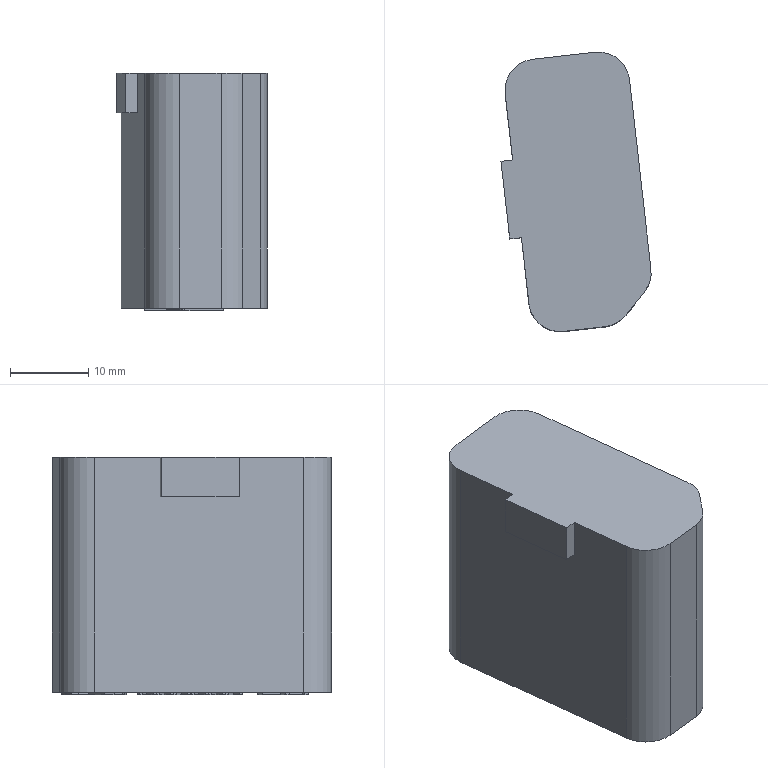Part | NX | features 13 2 | 1 solid | 132 faces | box 19.196 x 35.729 x 30.299 mm | volume 16184 mm3 | plane 101 | spline 24 | cylinder 7 | commonest cylinder face diameters 8 x5 21.767 x1 23.767 x1